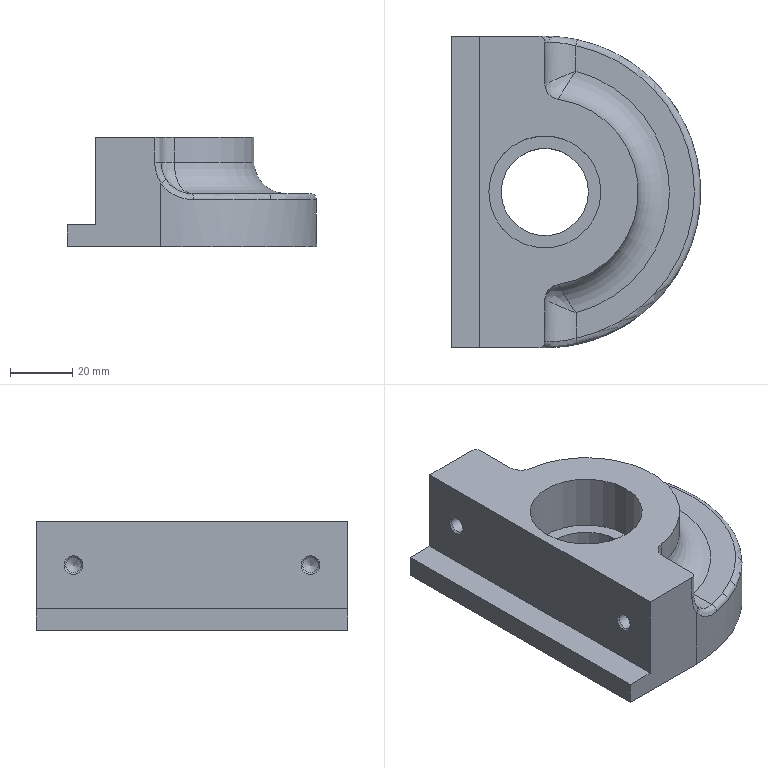Part | NX | features BLEND 3, DATUM_CSYS 2, EXTRUDE 2, HOLE PACKAGE 2, SIMPLE HOLE 2, SYMBOLIC_THREAD 2, BLOCK 1, CBORE_HOLE 1, DELETE FACE 1, SKETCH 1, SWP104 1 | 1 solid | 35 faces | box 80 x 100 x 35 mm | volume 145409 mm3 | cylinder 12 | plane 11 | spline 4 | torus 4 | cone 4 | commonest cylinder face diameters 4 x2 5 x2 10 x2 20 x2 28 x1 36 x1
STEP:
#1=CARTESIAN_POINT('',(0.,50.,0.));
#2=VERTEX_POINT('',#1);
#3=CARTESIAN_POINT('',(0.,50.,20.367));
#4=VERTEX_POINT('',#3);
#5=CARTESIAN_POINT('',(0.,50.,0.));
#6=DIRECTION('',(0.,0.,1.));
#7=VECTOR('',#6,1000.);
#8=LINE('',#5,#7);
#9=EDGE_CURVE('',#2,#4,#8,.T.);
#10=ORIENTED_EDGE('',*,*,#9,.T.);
#11=CARTESIAN_POINT('',(10.417,48.903,15.));
#12=VERTEX_POINT('',#11);
#13=CARTESIAN_POINT('',(0.,50.,20.367));
#14=CARTESIAN_POINT('',(1.172,50.,18.67));
#15=CARTESIAN_POINT('',(4.364,49.914,15.947));
#16=CARTESIAN_POINT('',(8.401,49.332,15.));
#17=CARTESIAN_POINT('',(10.417,48.903,15.));
#18=B_SPLINE_CURVE_WITH_KNOTS('',3,(#13,#14,#15,#16,#17),.UNSPECIFIED.,.F.,.F.,(4,1,4),(0.,0.006104,0.01221),.UNSPECIFIED.);
#19=EDGE_CURVE('',#4,#12,#18,.T.);
#20=ORIENTED_EDGE('',*,*,#19,.T.);
#21=CARTESIAN_POINT('',(10.417,-48.903,15.));
#22=VERTEX_POINT('',#21);
#23=CARTESIAN_POINT('',(0.,0.,15.));
#24=DIRECTION('',(0.,0.,1.));
#25=DIRECTION('',(1.,0.,0.));
#26=AXIS2_PLACEMENT_3D('',#23,#24,#25);
#27=CIRCLE('',#26,50.);
#28=EDGE_CURVE('',#12,#22,#27,.F.);
#29=ORIENTED_EDGE('',*,*,#28,.T.);
#30=CARTESIAN_POINT('',(0.,-50.,20.367));
#31=VERTEX_POINT('',#30);
#32=CARTESIAN_POINT('',(10.417,-48.903,15.));
#33=CARTESIAN_POINT('',(8.401,-49.332,15.));
#34=CARTESIAN_POINT('',(4.364,-49.914,15.947));
#35=CARTESIAN_POINT('',(1.172,-50.,18.67));
#36=CARTESIAN_POINT('',(0.,-50.,20.367));
#37=B_SPLINE_CURVE_WITH_KNOTS('',3,(#32,#33,#34,#35,#36),.UNSPECIFIED.,.F.,.F.,(4,1,4),(0.,0.006102,0.0122),.UNSPECIFIED.);
#38=EDGE_CURVE('',#22,#31,#37,.T.);
#39=ORIENTED_EDGE('',*,*,#38,.T.);
#40=CARTESIAN_POINT('',(0.,-50.,0.));
#41=VERTEX_POINT('',#40);
#42=CARTESIAN_POINT('',(0.,-50.,0.));
#43=DIRECTION('',(0.,0.,1.));
#44=VECTOR('',#43,1000.);
#45=LINE('',#42,#44);
#46=EDGE_CURVE('',#41,#31,#45,.T.);
#47=ORIENTED_EDGE('',*,*,#46,.F.);
#48=CARTESIAN_POINT('',(0.,0.,0.));
#49=DIRECTION('',(0.,0.,1.));
#50=DIRECTION('',(1.,0.,0.));
#51=AXIS2_PLACEMENT_3D('',#48,#49,#50);
#52=CIRCLE('',#51,50.);
#53=EDGE_CURVE('',#41,#2,#52,.T.);
#54=ORIENTED_EDGE('',*,*,#53,.T.);
#55=EDGE_LOOP('',(#10,#20,#29,#39,#47,#54));
#56=FACE_BOUND('',#55,.T.);
#57=CARTESIAN_POINT('',(0.,0.,0.));
#58=DIRECTION('',(0.,0.,1.));
#59=DIRECTION('',(1.,0.,0.));
#60=AXIS2_PLACEMENT_3D('',#57,#58,#59);
#61=CYLINDRICAL_SURFACE('',#60,50.);
#62=ADVANCED_FACE('',(#56),#61,.T.);
#63=CARTESIAN_POINT('',(-18.,0.,35.));
#64=VERTEX_POINT('',#63);
#65=CARTESIAN_POINT('',(0.,0.,35.));
#66=DIRECTION('',(0.,0.,-1.));
#67=DIRECTION('',(-1.,0.,0.));
#68=AXIS2_PLACEMENT_3D('',#65,#66,#67);
#69=CIRCLE('',#68,18.);
#70=EDGE_CURVE('',#64,#64,#69,.T.);
#71=ORIENTED_EDGE('',*,*,#70,.T.);
#72=EDGE_LOOP('',(#71));
#73=FACE_BOUND('',#72,.T.);
#74=CARTESIAN_POINT('',(-2.,-50.,35.));
#75=VERTEX_POINT('',#74);
#76=CARTESIAN_POINT('',(-21.,-50.,35.));
#77=VERTEX_POINT('',#76);
#78=CARTESIAN_POINT('',(-15.,-50.,35.));
#79=DIRECTION('',(-1.,0.,0.));
#80=VECTOR('',#79,1000.);
#81=LINE('',#78,#80);
#82=EDGE_CURVE('',#75,#77,#81,.T.);
#83=ORIENTED_EDGE('',*,*,#82,.F.);
#84=CARTESIAN_POINT('',(0.,-48.,35.));
#85=VERTEX_POINT('',#84);
#86=CARTESIAN_POINT('',(-2.,-48.,35.));
#87=DIRECTION('',(0.,0.,1.));
#88=DIRECTION('',(1.,0.,0.));
#89=AXIS2_PLACEMENT_3D('',#86,#87,#88);
#90=CIRCLE('',#89,2.);
#91=EDGE_CURVE('',#75,#85,#90,.T.);
#92=ORIENTED_EDGE('',*,*,#91,.T.);
#93=CARTESIAN_POINT('',(0.,-34.641,35.));
#94=VERTEX_POINT('',#93);
#95=CARTESIAN_POINT('',(0.,-50.,35.));
#96=DIRECTION('',(0.,-1.,0.));
#97=VECTOR('',#96,1000.);
#98=LINE('',#95,#97);
#99=EDGE_CURVE('',#85,#94,#98,.F.);
#100=ORIENTED_EDGE('',*,*,#99,.T.);
#101=CARTESIAN_POINT('',(4.286,-29.692,35.));
#102=VERTEX_POINT('',#101);
#103=CARTESIAN_POINT('',(5.,-34.641,35.));
#104=DIRECTION('',(0.,0.,1.));
#105=DIRECTION('',(1.,0.,0.));
#106=AXIS2_PLACEMENT_3D('',#103,#104,#105);
#107=CIRCLE('',#106,5.);
#108=EDGE_CURVE('',#94,#102,#107,.F.);
#109=ORIENTED_EDGE('',*,*,#108,.T.);
#110=CARTESIAN_POINT('',(4.286,29.692,35.));
#111=VERTEX_POINT('',#110);
#112=CARTESIAN_POINT('',(0.,0.,35.));
#113=DIRECTION('',(0.,0.,-1.));
#114=DIRECTION('',(-1.,0.,0.));
#115=AXIS2_PLACEMENT_3D('',#112,#113,#114);
#116=CIRCLE('',#115,30.);
#117=EDGE_CURVE('',#111,#102,#116,.T.);
#118=ORIENTED_EDGE('',*,*,#117,.F.);
#119=CARTESIAN_POINT('',(0.,34.641,35.));
#120=VERTEX_POINT('',#119);
#121=CARTESIAN_POINT('',(5.,34.641,35.));
#122=DIRECTION('',(0.,0.,1.));
#123=DIRECTION('',(1.,0.,0.));
#124=AXIS2_PLACEMENT_3D('',#121,#122,#123);
#125=CIRCLE('',#124,5.);
#126=EDGE_CURVE('',#111,#120,#125,.F.);
#127=ORIENTED_EDGE('',*,*,#126,.T.);
#128=CARTESIAN_POINT('',(0.,48.,35.));
#129=VERTEX_POINT('',#128);
#130=CARTESIAN_POINT('',(0.,50.,35.));
#131=DIRECTION('',(0.,1.,0.));
#132=VECTOR('',#131,1000.);
#133=LINE('',#130,#132);
#134=EDGE_CURVE('',#129,#120,#133,.F.);
#135=ORIENTED_EDGE('',*,*,#134,.F.);
#136=CARTESIAN_POINT('',(-2.,50.,35.));
#137=VERTEX_POINT('',#136);
#138=CARTESIAN_POINT('',(-2.,48.,35.));
#139=DIRECTION('',(0.,0.,1.));
#140=DIRECTION('',(1.,0.,0.));
#141=AXIS2_PLACEMENT_3D('',#138,#139,#140);
#142=CIRCLE('',#141,2.);
#143=EDGE_CURVE('',#129,#137,#142,.T.);
#144=ORIENTED_EDGE('',*,*,#143,.T.);
#145=CARTESIAN_POINT('',(-21.,50.,35.));
#146=VERTEX_POINT('',#145);
#147=CARTESIAN_POINT('',(-15.,50.,35.));
#148=DIRECTION('',(1.,0.,0.));
#149=VECTOR('',#148,1000.);
#150=LINE('',#147,#149);
#151=EDGE_CURVE('',#146,#137,#150,.T.);
#152=ORIENTED_EDGE('',*,*,#151,.F.);
#153=CARTESIAN_POINT('',(-21.,50.,35.));
#154=DIRECTION('',(0.,1.,0.));
#155=VECTOR('',#154,1000.);
#156=LINE('',#153,#155);
#157=EDGE_CURVE('',#146,#77,#156,.F.);
#158=ORIENTED_EDGE('',*,*,#157,.T.);
#159=EDGE_LOOP('',(#83,#92,#100,#109,#118,#127,#135,#144,#152,#158));
#160=FACE_BOUND('',#159,.T.);
#161=CARTESIAN_POINT('',(-15.,0.,35.));
#162=DIRECTION('',(0.,0.,1.));
#163=DIRECTION('',(1.,0.,0.));
#164=AXIS2_PLACEMENT_3D('',#161,#162,#163);
#165=PLANE('',#164);
#166=ADVANCED_FACE('',(#73,#160),#165,.T.);
#167=CARTESIAN_POINT('',(-2.,-50.,27.));
#168=VERTEX_POINT('',#167);
#169=CARTESIAN_POINT('',(10.,-50.,27.));
#170=DIRECTION('',(0.,-1.,0.));
#171=DIRECTION('',(0.,0.,-1.));
#172=AXIS2_PLACEMENT_3D('',#169,#170,#171);
#173=CIRCLE('',#172,12.);
#174=EDGE_CURVE('',#31,#168,#173,.F.);
#175=ORIENTED_EDGE('',*,*,#174,.T.);
#176=CARTESIAN_POINT('',(-2.,-50.,0.));
#177=DIRECTION('',(0.,0.,1.));
#178=VECTOR('',#177,1000.);
#179=LINE('',#176,#178);
#180=EDGE_CURVE('',#168,#75,#179,.T.);
#181=ORIENTED_EDGE('',*,*,#180,.T.);
#182=ORIENTED_EDGE('',*,*,#82,.T.);
#183=CARTESIAN_POINT('',(-21.,-50.,7.));
#184=VERTEX_POINT('',#183);
#185=CARTESIAN_POINT('',(-21.,-50.,35.));
#186=DIRECTION('',(0.,0.,-1.));
#187=VECTOR('',#186,1000.);
#188=LINE('',#185,#187);
#189=EDGE_CURVE('',#77,#184,#188,.T.);
#190=ORIENTED_EDGE('',*,*,#189,.T.);
#191=CARTESIAN_POINT('',(-30.,-50.,7.));
#192=VERTEX_POINT('',#191);
#193=CARTESIAN_POINT('',(-30.,-50.,7.));
#194=DIRECTION('',(1.,0.,0.));
#195=VECTOR('',#194,1000.);
#196=LINE('',#193,#195);
#197=EDGE_CURVE('',#192,#184,#196,.T.);
#198=ORIENTED_EDGE('',*,*,#197,.F.);
#199=CARTESIAN_POINT('',(-30.,-50.,0.));
#200=VERTEX_POINT('',#199);
#201=CARTESIAN_POINT('',(-30.,-50.,0.));
#202=DIRECTION('',(0.,0.,1.));
#203=VECTOR('',#202,1000.);
#204=LINE('',#201,#203);
#205=EDGE_CURVE('',#200,#192,#204,.T.);
#206=ORIENTED_EDGE('',*,*,#205,.F.);
#207=CARTESIAN_POINT('',(-15.,-50.,0.));
#208=DIRECTION('',(1.,0.,0.));
#209=VECTOR('',#208,1000.);
#210=LINE('',#207,#209);
#211=EDGE_CURVE('',#200,#41,#210,.T.);
#212=ORIENTED_EDGE('',*,*,#211,.T.);
#213=ORIENTED_EDGE('',*,*,#46,.T.);
#214=EDGE_LOOP('',(#175,#181,#182,#190,#198,#206,#212,#213));
#215=FACE_BOUND('',#214,.T.);
#216=CARTESIAN_POINT('',(-15.,-50.,0.));
#217=DIRECTION('',(0.,-1.,0.));
#218=DIRECTION('',(0.,0.,-1.));
#219=AXIS2_PLACEMENT_3D('',#216,#217,#218);
#220=PLANE('',#219);
#221=ADVANCED_FACE('',(#215),#220,.T.);
#222=CARTESIAN_POINT('',(-30.,50.,7.));
#223=VERTEX_POINT('',#222);
#224=CARTESIAN_POINT('',(-30.,50.,7.));
#225=DIRECTION('',(0.,-1.,0.));
#226=VECTOR('',#225,1000.);
#227=LINE('',#224,#226);
#228=EDGE_CURVE('',#223,#192,#227,.T.);
#229=ORIENTED_EDGE('',*,*,#228,.F.);
#230=CARTESIAN_POINT('',(-30.,50.,0.));
#231=VERTEX_POINT('',#230);
#232=CARTESIAN_POINT('',(-30.,50.,0.));
#233=DIRECTION('',(0.,0.,1.));
#234=VECTOR('',#233,1000.);
#235=LINE('',#232,#234);
#236=EDGE_CURVE('',#231,#223,#235,.T.);
#237=ORIENTED_EDGE('',*,*,#236,.F.);
#238=CARTESIAN_POINT('',(-30.,0.,0.));
#239=DIRECTION('',(0.,-1.,0.));
#240=VECTOR('',#239,1000.);
#241=LINE('',#238,#240);
#242=EDGE_CURVE('',#231,#200,#241,.T.);
#243=ORIENTED_EDGE('',*,*,#242,.T.);
#244=ORIENTED_EDGE('',*,*,#205,.T.);
#245=EDGE_LOOP('',(#229,#237,#243,#244));
#246=FACE_BOUND('',#245,.T.);
#247=CARTESIAN_POINT('',(-30.,0.,0.));
#248=DIRECTION('',(-1.,0.,0.));
#249=DIRECTION('',(0.,0.,1.));
#250=AXIS2_PLACEMENT_3D('',#247,#248,#249);
#251=PLANE('',#250);
#252=ADVANCED_FACE('',(#246),#251,.T.);
#253=ORIENTED_EDGE('',*,*,#151,.T.);
#254=CARTESIAN_POINT('',(-2.,50.,27.));
#255=VERTEX_POINT('',#254);
#256=CARTESIAN_POINT('',(-2.,50.,0.));
#257=DIRECTION('',(0.,0.,-1.));
#258=VECTOR('',#257,1000.);
#259=LINE('',#256,#258);
#260=EDGE_CURVE('',#137,#255,#259,.T.);
#261=ORIENTED_EDGE('',*,*,#260,.T.);
#262=CARTESIAN_POINT('',(10.,50.,27.));
#263=DIRECTION('',(0.,1.,0.));
#264=DIRECTION('',(0.,0.,1.));
#265=AXIS2_PLACEMENT_3D('',#262,#263,#264);
#266=CIRCLE('',#265,12.);
#267=EDGE_CURVE('',#255,#4,#266,.F.);
#268=ORIENTED_EDGE('',*,*,#267,.T.);
#269=ORIENTED_EDGE('',*,*,#9,.F.);
#270=CARTESIAN_POINT('',(-15.,50.,0.));
#271=DIRECTION('',(-1.,0.,0.));
#272=VECTOR('',#271,1000.);
#273=LINE('',#270,#272);
#274=EDGE_CURVE('',#2,#231,#273,.T.);
#275=ORIENTED_EDGE('',*,*,#274,.T.);
#276=ORIENTED_EDGE('',*,*,#236,.T.);
#277=CARTESIAN_POINT('',(-21.,50.,7.));
#278=VERTEX_POINT('',#277);
#279=CARTESIAN_POINT('',(-30.,50.,7.));
#280=DIRECTION('',(1.,0.,0.));
#281=VECTOR('',#280,1000.);
#282=LINE('',#279,#281);
#283=EDGE_CURVE('',#223,#278,#282,.T.);
#284=ORIENTED_EDGE('',*,*,#283,.T.);
#285=CARTESIAN_POINT('',(-21.,50.,35.));
#286=DIRECTION('',(0.,0.,-1.));
#287=VECTOR('',#286,1000.);
#288=LINE('',#285,#287);
#289=EDGE_CURVE('',#146,#278,#288,.T.);
#290=ORIENTED_EDGE('',*,*,#289,.F.);
#291=EDGE_LOOP('',(#253,#261,#268,#269,#275,#276,#284,#290));
#292=FACE_BOUND('',#291,.T.);
#293=CARTESIAN_POINT('',(-15.,50.,0.));
#294=DIRECTION('',(0.,1.,0.));
#295=DIRECTION('',(0.,0.,1.));
#296=AXIS2_PLACEMENT_3D('',#293,#294,#295);
#297=PLANE('',#296);
#298=ADVANCED_FACE('',(#292),#297,.T.);
#299=CARTESIAN_POINT('',(-14.,0.,0.));
#300=VERTEX_POINT('',#299);
#301=CARTESIAN_POINT('',(0.,0.,0.));
#302=DIRECTION('',(0.,0.,-1.));
#303=DIRECTION('',(-1.,0.,0.));
#304=AXIS2_PLACEMENT_3D('',#301,#302,#303);
#305=CIRCLE('',#304,14.);
#306=EDGE_CURVE('',#300,#300,#305,.T.);
#307=ORIENTED_EDGE('',*,*,#306,.F.);
#308=EDGE_LOOP('',(#307));
#309=FACE_BOUND('',#308,.T.);
#310=ORIENTED_EDGE('',*,*,#211,.F.);
#311=ORIENTED_EDGE('',*,*,#242,.F.);
#312=ORIENTED_EDGE('',*,*,#274,.F.);
#313=ORIENTED_EDGE('',*,*,#53,.F.);
#314=EDGE_LOOP('',(#310,#311,#312,#313));
#315=FACE_BOUND('',#314,.T.);
#316=CARTESIAN_POINT('',(-15.,0.,0.));
#317=DIRECTION('',(0.,0.,-1.));
#318=DIRECTION('',(-1.,0.,0.));
#319=AXIS2_PLACEMENT_3D('',#316,#317,#318);
#320=PLANE('',#319);
#321=ADVANCED_FACE('',(#309,#315),#320,.T.);
#322=ORIENTED_EDGE('',*,*,#197,.T.);
#323=CARTESIAN_POINT('',(-21.,50.,7.));
#324=DIRECTION('',(0.,1.,0.));
#325=VECTOR('',#324,1000.);
#326=LINE('',#323,#325);
#327=EDGE_CURVE('',#184,#278,#326,.T.);
#328=ORIENTED_EDGE('',*,*,#327,.T.);
#329=ORIENTED_EDGE('',*,*,#283,.F.);
#330=ORIENTED_EDGE('',*,*,#228,.T.);
#331=EDGE_LOOP('',(#322,#328,#329,#330));
#332=FACE_BOUND('',#331,.T.);
#333=CARTESIAN_POINT('',(-30.,50.,7.));
#334=DIRECTION('',(0.,0.,1.));
#335=DIRECTION('',(0.,-1.,0.));
#336=AXIS2_PLACEMENT_3D('',#333,#334,#335);
#337=PLANE('',#336);
#338=ADVANCED_FACE('',(#332),#337,.T.);
#339=CARTESIAN_POINT('',(-21.,38.,18.));
#340=VERTEX_POINT('',#339);
#341=CARTESIAN_POINT('',(-21.,38.,21.));
#342=DIRECTION('',(1.,0.,0.));
#343=DIRECTION('',(0.,0.,-1.));
#344=AXIS2_PLACEMENT_3D('',#341,#342,#343);
#345=CIRCLE('',#344,3.);
#346=EDGE_CURVE('',#340,#340,#345,.T.);
#347=ORIENTED_EDGE('',*,*,#346,.T.);
#348=EDGE_LOOP('',(#347));
#349=FACE_BOUND('',#348,.T.);
#350=CARTESIAN_POINT('',(-21.,-38.,18.));
#351=VERTEX_POINT('',#350);
#352=CARTESIAN_POINT('',(-21.,-38.,21.));
#353=DIRECTION('',(1.,0.,0.));
#354=DIRECTION('',(0.,0.,-1.));
#355=AXIS2_PLACEMENT_3D('',#352,#353,#354);
#356=CIRCLE('',#355,3.);
#357=EDGE_CURVE('',#351,#351,#356,.T.);
#358=ORIENTED_EDGE('',*,*,#357,.T.);
#359=EDGE_LOOP('',(#358));
#360=FACE_BOUND('',#359,.T.);
#361=ORIENTED_EDGE('',*,*,#327,.F.);
#362=ORIENTED_EDGE('',*,*,#189,.F.);
#363=ORIENTED_EDGE('',*,*,#157,.F.);
#364=ORIENTED_EDGE('',*,*,#289,.T.);
#365=EDGE_LOOP('',(#361,#362,#363,#364));
#366=FACE_BOUND('',#365,.T.);
#367=CARTESIAN_POINT('',(-21.,50.,35.));
#368=DIRECTION('',(1.,0.,0.));
#369=DIRECTION('',(0.,0.,-1.));
#370=AXIS2_PLACEMENT_3D('',#367,#368,#369);
#371=PLANE('',#370);
#372=ADVANCED_FACE('',(#349,#360,#366),#371,.F.);
#373=ORIENTED_EDGE('',*,*,#99,.F.);
#374=CARTESIAN_POINT('',(0.,-48.,27.));
#375=VERTEX_POINT('',#374);
#376=CARTESIAN_POINT('',(0.,-48.,26.));
#377=DIRECTION('',(0.,0.,-1.));
#378=VECTOR('',#377,1000.);
#379=LINE('',#376,#378);
#380=EDGE_CURVE('',#85,#375,#379,.T.);
#381=ORIENTED_EDGE('',*,*,#380,.T.);
#382=CARTESIAN_POINT('',(0.,-34.641,27.));
#383=VERTEX_POINT('',#382);
#384=CARTESIAN_POINT('',(0.,-34.641,27.));
#385=DIRECTION('',(0.,-1.,0.));
#386=VECTOR('',#385,1000.);
#387=LINE('',#384,#386);
#388=EDGE_CURVE('',#375,#383,#387,.F.);
#389=ORIENTED_EDGE('',*,*,#388,.T.);
#390=CARTESIAN_POINT('',(0.,-34.641,35.));
#391=DIRECTION('',(0.,0.,-1.));
#392=VECTOR('',#391,1000.);
#393=LINE('',#390,#392);
#394=EDGE_CURVE('',#383,#94,#393,.F.);
#395=ORIENTED_EDGE('',*,*,#394,.T.);
#396=EDGE_LOOP('',(#373,#381,#389,#395));
#397=FACE_BOUND('',#396,.T.);
#398=CARTESIAN_POINT('',(0.,-50.,26.));
#399=DIRECTION('',(-1.,0.,0.));
#400=DIRECTION('',(0.,0.,-1.));
#401=AXIS2_PLACEMENT_3D('',#398,#399,#400);
#402=PLANE('',#401);
#403=ADVANCED_FACE('',(#397),#402,.F.);
#404=CARTESIAN_POINT('',(10.,-38.73,17.));
#405=VERTEX_POINT('',#404);
#406=CARTESIAN_POINT('',(10.,-46.947,17.));
#407=VERTEX_POINT('',#406);
#408=CARTESIAN_POINT('',(10.,-50.,17.));
#409=DIRECTION('',(0.,1.,0.));
#410=VECTOR('',#409,1000.);
#411=LINE('',#408,#410);
#412=EDGE_CURVE('',#405,#407,#411,.F.);
#413=ORIENTED_EDGE('',*,*,#412,.T.);
#414=CARTESIAN_POINT('',(10.,46.947,17.));
#415=VERTEX_POINT('',#414);
#416=CARTESIAN_POINT('',(0.,0.,17.));
#417=DIRECTION('',(0.,0.,1.));
#418=DIRECTION('',(1.,0.,0.));
#419=AXIS2_PLACEMENT_3D('',#416,#417,#418);
#420=CIRCLE('',#419,48.);
#421=EDGE_CURVE('',#407,#415,#420,.T.);
#422=ORIENTED_EDGE('',*,*,#421,.T.);
#423=CARTESIAN_POINT('',(10.,38.73,17.));
#424=VERTEX_POINT('',#423);
#425=CARTESIAN_POINT('',(10.,34.641,17.));
#426=DIRECTION('',(0.,1.,0.));
#427=VECTOR('',#426,1000.);
#428=LINE('',#425,#427);
#429=EDGE_CURVE('',#415,#424,#428,.F.);
#430=ORIENTED_EDGE('',*,*,#429,.T.);
#431=CARTESIAN_POINT('',(0.,0.,17.));
#432=DIRECTION('',(0.,0.,1.));
#433=DIRECTION('',(1.,0.,0.));
#434=AXIS2_PLACEMENT_3D('',#431,#432,#433);
#435=CIRCLE('',#434,40.);
#436=EDGE_CURVE('',#424,#405,#435,.F.);
#437=ORIENTED_EDGE('',*,*,#436,.T.);
#438=EDGE_LOOP('',(#413,#422,#430,#437));
#439=FACE_BOUND('',#438,.T.);
#440=CARTESIAN_POINT('',(0.,0.,17.));
#441=DIRECTION('',(0.,0.,1.));
#442=DIRECTION('',(1.,0.,0.));
#443=AXIS2_PLACEMENT_3D('',#440,#441,#442);
#444=PLANE('',#443);
#445=ADVANCED_FACE('',(#439),#444,.T.);
#446=CARTESIAN_POINT('',(0.,34.641,27.));
#447=VERTEX_POINT('',#446);
#448=CARTESIAN_POINT('',(0.,48.,27.));
#449=VERTEX_POINT('',#448);
#450=CARTESIAN_POINT('',(0.,50.,27.));
#451=DIRECTION('',(0.,1.,0.));
#452=VECTOR('',#451,1000.);
#453=LINE('',#450,#452);
#454=EDGE_CURVE('',#447,#449,#453,.T.);
#455=ORIENTED_EDGE('',*,*,#454,.T.);
#456=CARTESIAN_POINT('',(0.,48.,26.));
#457=DIRECTION('',(0.,0.,-1.));
#458=VECTOR('',#457,1000.);
#459=LINE('',#456,#458);
#460=EDGE_CURVE('',#449,#129,#459,.F.);
#461=ORIENTED_EDGE('',*,*,#460,.T.);
#462=ORIENTED_EDGE('',*,*,#134,.T.);
#463=CARTESIAN_POINT('',(0.,34.641,17.));
#464=DIRECTION('',(0.,0.,1.));
#465=VECTOR('',#464,1000.);
#466=LINE('',#463,#465);
#467=EDGE_CURVE('',#120,#447,#466,.F.);
#468=ORIENTED_EDGE('',*,*,#467,.T.);
#469=EDGE_LOOP('',(#455,#461,#462,#468));
#470=FACE_BOUND('',#469,.T.);
#471=CARTESIAN_POINT('',(0.,50.,26.));
#472=DIRECTION('',(1.,0.,0.));
#473=DIRECTION('',(0.,0.,-1.));
#474=AXIS2_PLACEMENT_3D('',#471,#472,#473);
#475=PLANE('',#474);
#476=ADVANCED_FACE('',(#470),#475,.T.);
#477=CARTESIAN_POINT('',(4.286,-29.692,27.));
#478=VERTEX_POINT('',#477);
#479=CARTESIAN_POINT('',(4.286,-29.692,35.));
#480=DIRECTION('',(0.,0.,-1.));
#481=VECTOR('',#480,1000.);
#482=LINE('',#479,#481);
#483=EDGE_CURVE('',#102,#478,#482,.T.);
#484=ORIENTED_EDGE('',*,*,#483,.T.);
#485=CARTESIAN_POINT('',(4.286,29.692,27.));
#486=VERTEX_POINT('',#485);
#487=CARTESIAN_POINT('',(0.,0.,27.));
#488=DIRECTION('',(0.,0.,1.));
#489=DIRECTION('',(1.,0.,0.));
#490=AXIS2_PLACEMENT_3D('',#487,#488,#489);
#491=CIRCLE('',#490,30.);
#492=EDGE_CURVE('',#478,#486,#491,.T.);
#493=ORIENTED_EDGE('',*,*,#492,.T.);
#494=CARTESIAN_POINT('',(4.286,29.692,35.));
#495=DIRECTION('',(0.,0.,-1.));
#496=VECTOR('',#495,1000.);
#497=LINE('',#494,#496);
#498=EDGE_CURVE('',#486,#111,#497,.F.);
#499=ORIENTED_EDGE('',*,*,#498,.T.);
#500=ORIENTED_EDGE('',*,*,#117,.T.);
#501=EDGE_LOOP('',(#484,#493,#499,#500));
#502=FACE_BOUND('',#501,.T.);
#503=CARTESIAN_POINT('',(0.,0.,35.));
#504=DIRECTION('',(0.,0.,-1.));
#505=DIRECTION('',(-1.,0.,0.));
#506=AXIS2_PLACEMENT_3D('',#503,#504,#505);
#507=CYLINDRICAL_SURFACE('',#506,30.);
#508=ADVANCED_FACE('',(#502),#507,.T.);
#509=ORIENTED_EDGE('',*,*,#306,.T.);
#510=EDGE_LOOP('',(#509));
#511=FACE_BOUND('',#510,.T.);
#512=CARTESIAN_POINT('',(-14.,0.,17.));
#513=VERTEX_POINT('',#512);
#514=CARTESIAN_POINT('',(0.,0.,17.));
#515=DIRECTION('',(0.,0.,-1.));
#516=DIRECTION('',(-1.,0.,0.));
#517=AXIS2_PLACEMENT_3D('',#514,#515,#516);
#518=CIRCLE('',#517,14.);
#519=EDGE_CURVE('',#513,#513,#518,.F.);
#520=ORIENTED_EDGE('',*,*,#519,.T.);
#521=EDGE_LOOP('',(#520));
#522=FACE_BOUND('',#521,.T.);
#523=CARTESIAN_POINT('',(0.,0.,-54.83));
#524=DIRECTION('',(0.,0.,-1.));
#525=DIRECTION('',(-1.,0.,0.));
#526=AXIS2_PLACEMENT_3D('',#523,#524,#525);
#527=CYLINDRICAL_SURFACE('',#526,14.);
#528=ADVANCED_FACE('',(#511,#522),#527,.F.);
#529=ORIENTED_EDGE('',*,*,#519,.F.);
#530=EDGE_LOOP('',(#529));
#531=FACE_BOUND('',#530,.T.);
#532=CARTESIAN_POINT('',(-18.,0.,17.));
#533=VERTEX_POINT('',#532);
#534=CARTESIAN_POINT('',(0.,0.,17.));
#535=DIRECTION('',(0.,0.,-1.));
#536=DIRECTION('',(-1.,0.,0.));
#537=AXIS2_PLACEMENT_3D('',#534,#535,#536);
#538=CIRCLE('',#537,18.);
#539=EDGE_CURVE('',#533,#533,#538,.F.);
#540=ORIENTED_EDGE('',*,*,#539,.T.);
#541=EDGE_LOOP('',(#540));
#542=FACE_BOUND('',#541,.T.);
#543=CARTESIAN_POINT('',(0.,0.,17.));
#544=DIRECTION('',(0.,0.,-1.));
#545=DIRECTION('',(-1.,0.,0.));
#546=AXIS2_PLACEMENT_3D('',#543,#544,#545);
#547=PLANE('',#546);
#548=ADVANCED_FACE('',(#531,#542),#547,.F.);
#549=ORIENTED_EDGE('',*,*,#539,.F.);
#550=EDGE_LOOP('',(#549));
#551=FACE_BOUND('',#550,.T.);
#552=ORIENTED_EDGE('',*,*,#70,.F.);
#553=EDGE_LOOP('',(#552));
#554=FACE_BOUND('',#553,.T.);
#555=CARTESIAN_POINT('',(0.,0.,35.));
#556=DIRECTION('',(0.,0.,-1.));
#557=DIRECTION('',(-1.,0.,0.));
#558=AXIS2_PLACEMENT_3D('',#555,#556,#557);
#559=CYLINDRICAL_SURFACE('',#558,18.);
#560=ADVANCED_FACE('',(#551,#554),#559,.F.);
#561=ORIENTED_EDGE('',*,*,#394,.F.);
#562=CARTESIAN_POINT('',(5.,-34.641,27.));
#563=DIRECTION('',(0.,0.,-1.));
#564=DIRECTION('',(-1.,0.,0.));
#565=AXIS2_PLACEMENT_3D('',#562,#563,#564);
#566=CIRCLE('',#565,5.);
#567=EDGE_CURVE('',#383,#478,#566,.T.);
#568=ORIENTED_EDGE('',*,*,#567,.T.);
#569=ORIENTED_EDGE('',*,*,#483,.F.);
#570=ORIENTED_EDGE('',*,*,#108,.F.);
#571=EDGE_LOOP('',(#561,#568,#569,#570));
#572=FACE_BOUND('',#571,.T.);
#573=CARTESIAN_POINT('',(5.,-34.641,35.));
#574=DIRECTION('',(0.,0.,-1.));
#575=DIRECTION('',(-1.,0.,0.));
#576=AXIS2_PLACEMENT_3D('',#573,#574,#575);
#577=CYLINDRICAL_SURFACE('',#576,5.);
#578=ADVANCED_FACE('',(#572),#577,.F.);
#579=ORIENTED_EDGE('',*,*,#498,.F.);
#580=CARTESIAN_POINT('',(5.,34.641,27.));
#581=DIRECTION('',(0.,0.,-1.));
#582=DIRECTION('',(-1.,0.,0.));
#583=AXIS2_PLACEMENT_3D('',#580,#581,#582);
#584=CIRCLE('',#583,5.);
#585=EDGE_CURVE('',#486,#447,#584,.T.);
#586=ORIENTED_EDGE('',*,*,#585,.T.);
#587=ORIENTED_EDGE('',*,*,#467,.F.);
#588=ORIENTED_EDGE('',*,*,#126,.F.);
#589=EDGE_LOOP('',(#579,#586,#587,#588));
#590=FACE_BOUND('',#589,.T.);
#591=CARTESIAN_POINT('',(5.,34.641,35.));
#592=DIRECTION('',(0.,0.,-1.));
#593=DIRECTION('',(-1.,0.,0.));
#594=AXIS2_PLACEMENT_3D('',#591,#592,#593);
#595=CYLINDRICAL_SURFACE('',#594,5.);
#596=ADVANCED_FACE('',(#590),#595,.F.);
#597=ORIENTED_EDGE('',*,*,#429,.F.);
#598=CARTESIAN_POINT('',(1.667,48.,21.472));
#599=VERTEX_POINT('',#598);
#600=CARTESIAN_POINT('',(10.,46.947,17.));
#601=CARTESIAN_POINT('',(8.381,47.361,17.));
#602=CARTESIAN_POINT('',(5.123,47.922,17.803));
#603=CARTESIAN_POINT('',(2.591,48.,20.079));
#604=CARTESIAN_POINT('',(1.667,48.,21.472));
#605=B_SPLINE_CURVE_WITH_KNOTS('',3,(#600,#601,#602,#603,#604),.UNSPECIFIED.,.F.,.F.,(4,1,4),(0.,0.004943,0.009887),.UNSPECIFIED.);
#606=EDGE_CURVE('',#415,#599,#605,.T.);
#607=ORIENTED_EDGE('',*,*,#606,.T.);
#608=CARTESIAN_POINT('',(10.,48.,27.));
#609=DIRECTION('',(0.,1.,0.));
#610=DIRECTION('',(0.,0.,1.));
#611=AXIS2_PLACEMENT_3D('',#608,#609,#610);
#612=CIRCLE('',#611,10.);
#613=EDGE_CURVE('',#599,#449,#612,.T.);
#614=ORIENTED_EDGE('',*,*,#613,.T.);
#615=ORIENTED_EDGE('',*,*,#454,.F.);
#616=CARTESIAN_POINT('',(0.,34.641,27.));
#617=CARTESIAN_POINT('',(0.,34.641,24.256));
#618=CARTESIAN_POINT('',(2.37,35.682,18.987));
#619=CARTESIAN_POINT('',(7.47,37.75,17.));
#620=CARTESIAN_POINT('',(10.,38.73,17.));
#621=B_SPLINE_CURVE_WITH_KNOTS('',3,(#616,#617,#618,#619,#620),.UNSPECIFIED.,.F.,.F.,(4,1,4),(0.,0.008138,0.01628),.UNSPECIFIED.);
#622=EDGE_CURVE('',#424,#447,#621,.F.);
#623=ORIENTED_EDGE('',*,*,#622,.F.);
#624=EDGE_LOOP('',(#597,#607,#614,#615,#623));
#625=FACE_BOUND('',#624,.T.);
#626=CARTESIAN_POINT('',(10.,50.,27.));
#627=DIRECTION('',(0.,-1.,0.));
#628=DIRECTION('',(1.,0.,0.));
#629=AXIS2_PLACEMENT_3D('',#626,#627,#628);
#630=CYLINDRICAL_SURFACE('',#629,10.);
#631=ADVANCED_FACE('',(#625),#630,.F.);
#632=ORIENTED_EDGE('',*,*,#622,.T.);
#633=ORIENTED_EDGE('',*,*,#585,.F.);
#634=CARTESIAN_POINT('',(4.286,29.692,27.));
#635=CARTESIAN_POINT('',(4.286,29.692,24.268));
#636=CARTESIAN_POINT('',(5.451,31.92,18.989));
#637=CARTESIAN_POINT('',(8.426,36.534,17.));
#638=CARTESIAN_POINT('',(10.,38.73,17.));
#639=B_SPLINE_CURVE_WITH_KNOTS('',3,(#634,#635,#636,#637,#638),.UNSPECIFIED.,.F.,.F.,(4,1,4),(0.,0.008105,0.01621),.UNSPECIFIED.);
#640=EDGE_CURVE('',#424,#486,#639,.F.);
#641=ORIENTED_EDGE('',*,*,#640,.F.);
#642=EDGE_LOOP('',(#632,#633,#641));
#643=FACE_BOUND('',#642,.T.);
#644=CARTESIAN_POINT('',(0.,34.641,27.));
#645=CARTESIAN_POINT('',(0.,30.311,27.));
#646=CARTESIAN_POINT('',(4.286,29.692,27.));
#647=CARTESIAN_POINT('',(0.,34.641,26.239));
#648=CARTESIAN_POINT('',(0.000000013,30.311,25.953));
#649=CARTESIAN_POINT('',(4.286,29.692,26.239));
#650=CARTESIAN_POINT('',(0.1714,34.715,24.752));
#651=CARTESIAN_POINT('',(0.2998,30.58,23.954));
#652=CARTESIAN_POINT('',(4.373,29.853,24.752));
#653=CARTESIAN_POINT('',(1.144,35.135,21.978));
#654=CARTESIAN_POINT('',(1.779,31.901,20.752));
#655=CARTESIAN_POINT('',(4.874,30.762,21.978));
#656=CARTESIAN_POINT('',(3.245,36.025,19.304));
#657=CARTESIAN_POINT('',(4.201,34.022,18.526));
#658=CARTESIAN_POINT('',(5.994,32.706,19.304));
#659=CARTESIAN_POINT('',(6.439,37.334,17.426));
#660=CARTESIAN_POINT('',(7.079,36.429,17.269));
#661=CARTESIAN_POINT('',(7.815,35.599,17.426));
#662=CARTESIAN_POINT('',(8.816,38.271,17.));
#663=CARTESIAN_POINT('',(9.038,37.985,17.));
#664=CARTESIAN_POINT('',(9.26,37.698,17.));
#665=CARTESIAN_POINT('',(10.,38.73,17.));
#666=CARTESIAN_POINT('',(10.,38.73,17.));
#667=CARTESIAN_POINT('',(10.,38.73,17.));
#668=(BOUNDED_SURFACE()B_SPLINE_SURFACE(3,2,((#644,#645,#646),(#647,#648,#649),(#650,#651,#652),(#653,#654,#655),(#656,#657,#658),(#659,#660,#661),(#662,#663,#664),(#665,#666,#667)),.UNSPECIFIED.,.F.,.F.,.F.)B_SPLINE_SURFACE_WITH_KNOTS((4,1,1,1,1,4),(3,3),(0.,0.001123,0.002246,0.004492,0.006738,0.008984),(0.,1.),.UNSPECIFIED.)GEOMETRIC_REPRESENTATION_ITEM()RATIONAL_B_SPLINE_SURFACE(((1.,0.7559,1.),(1.,0.7559,1.),(1.,0.7666,1.),(1.,0.8212,1.),(1.,0.9112,1.),(1.,0.9837,1.),(1.,1.,1.),(1.,1.,1.)))REPRESENTATION_ITEM('')SURFACE());
#669=ADVANCED_FACE('',(#643),#668,.F.);
#670=ORIENTED_EDGE('',*,*,#640,.T.);
#671=ORIENTED_EDGE('',*,*,#492,.F.);
#672=CARTESIAN_POINT('',(4.286,-29.692,27.));
#673=CARTESIAN_POINT('',(4.286,-29.692,24.268));
#674=CARTESIAN_POINT('',(5.451,-31.92,18.989));
#675=CARTESIAN_POINT('',(8.426,-36.534,17.));
#676=CARTESIAN_POINT('',(10.,-38.73,17.));
#677=B_SPLINE_CURVE_WITH_KNOTS('',3,(#672,#673,#674,#675,#676),.UNSPECIFIED.,.F.,.F.,(4,1,4),(0.,0.008105,0.01621),.UNSPECIFIED.);
#678=EDGE_CURVE('',#405,#478,#677,.F.);
#679=ORIENTED_EDGE('',*,*,#678,.F.);
#680=ORIENTED_EDGE('',*,*,#436,.F.);
#681=EDGE_LOOP('',(#670,#671,#679,#680));
#682=FACE_BOUND('',#681,.T.);
#683=CARTESIAN_POINT('',(0.,0.,27.));
#684=DIRECTION('',(0.,0.,1.));
#685=DIRECTION('',(1.,0.,0.));
#686=AXIS2_PLACEMENT_3D('',#683,#684,#685);
#687=TOROIDAL_SURFACE('',#686,40.,10.);
#688=ADVANCED_FACE('',(#682),#687,.F.);
#689=ORIENTED_EDGE('',*,*,#678,.T.);
#690=ORIENTED_EDGE('',*,*,#567,.F.);
#691=CARTESIAN_POINT('',(0.,-34.641,27.));
#692=CARTESIAN_POINT('',(0.,-34.641,24.256));
#693=CARTESIAN_POINT('',(2.37,-35.682,18.987));
#694=CARTESIAN_POINT('',(7.47,-37.75,17.));
#695=CARTESIAN_POINT('',(10.,-38.73,17.));
#696=B_SPLINE_CURVE_WITH_KNOTS('',3,(#691,#692,#693,#694,#695),.UNSPECIFIED.,.F.,.F.,(4,1,4),(0.,0.008138,0.01628),.UNSPECIFIED.);
#697=EDGE_CURVE('',#405,#383,#696,.F.);
#698=ORIENTED_EDGE('',*,*,#697,.F.);
#699=EDGE_LOOP('',(#689,#690,#698));
#700=FACE_BOUND('',#699,.T.);
#701=CARTESIAN_POINT('',(4.286,-29.692,27.));
#702=CARTESIAN_POINT('',(0.,-30.311,27.));
#703=CARTESIAN_POINT('',(0.,-34.641,27.));
#704=CARTESIAN_POINT('',(4.286,-29.692,26.239));
#705=CARTESIAN_POINT('',(0.000000013,-30.311,25.953));
#706=CARTESIAN_POINT('',(0.,-34.641,26.239));
#707=CARTESIAN_POINT('',(4.373,-29.853,24.752));
#708=CARTESIAN_POINT('',(0.2998,-30.58,23.954));
#709=CARTESIAN_POINT('',(0.1714,-34.715,24.752));
#710=CARTESIAN_POINT('',(4.874,-30.762,21.978));
#711=CARTESIAN_POINT('',(1.779,-31.901,20.752));
#712=CARTESIAN_POINT('',(1.144,-35.135,21.978));
#713=CARTESIAN_POINT('',(5.994,-32.706,19.304));
#714=CARTESIAN_POINT('',(4.201,-34.022,18.526));
#715=CARTESIAN_POINT('',(3.245,-36.025,19.304));
#716=CARTESIAN_POINT('',(7.815,-35.599,17.426));
#717=CARTESIAN_POINT('',(7.079,-36.429,17.269));
#718=CARTESIAN_POINT('',(6.439,-37.334,17.426));
#719=CARTESIAN_POINT('',(9.26,-37.698,17.));
#720=CARTESIAN_POINT('',(9.038,-37.985,17.));
#721=CARTESIAN_POINT('',(8.816,-38.271,17.));
#722=CARTESIAN_POINT('',(10.,-38.73,17.));
#723=CARTESIAN_POINT('',(10.,-38.73,17.));
#724=CARTESIAN_POINT('',(10.,-38.73,17.));
#725=(BOUNDED_SURFACE()B_SPLINE_SURFACE(3,2,((#701,#702,#703),(#704,#705,#706),(#707,#708,#709),(#710,#711,#712),(#713,#714,#715),(#716,#717,#718),(#719,#720,#721),(#722,#723,#724)),.UNSPECIFIED.,.F.,.F.,.F.)B_SPLINE_SURFACE_WITH_KNOTS((4,1,1,1,1,4),(3,3),(0.,0.001123,0.002246,0.004492,0.006738,0.008984),(0.,1.),.UNSPECIFIED.)GEOMETRIC_REPRESENTATION_ITEM()RATIONAL_B_SPLINE_SURFACE(((1.,0.7559,1.),(1.,0.7559,1.),(1.,0.7666,1.),(1.,0.8212,1.),(1.,0.9112,1.),(1.,0.9837,1.),(1.,1.,1.),(1.,1.,1.)))REPRESENTATION_ITEM('')SURFACE());
#726=ADVANCED_FACE('',(#700),#725,.F.);
#727=ORIENTED_EDGE('',*,*,#388,.F.);
#728=CARTESIAN_POINT('',(1.667,-48.,21.472));
#729=VERTEX_POINT('',#728);
#730=CARTESIAN_POINT('',(10.,-48.,27.));
#731=DIRECTION('',(0.,-1.,0.));
#732=DIRECTION('',(0.,0.,-1.));
#733=AXIS2_PLACEMENT_3D('',#730,#731,#732);
#734=CIRCLE('',#733,10.);
#735=EDGE_CURVE('',#375,#729,#734,.T.);
#736=ORIENTED_EDGE('',*,*,#735,.T.);
#737=CARTESIAN_POINT('',(1.667,-48.,21.472));
#738=CARTESIAN_POINT('',(2.591,-48.,20.079));
#739=CARTESIAN_POINT('',(5.123,-47.922,17.803));
#740=CARTESIAN_POINT('',(8.381,-47.361,17.));
#741=CARTESIAN_POINT('',(10.,-46.947,17.));
#742=B_SPLINE_CURVE_WITH_KNOTS('',3,(#737,#738,#739,#740,#741),.UNSPECIFIED.,.F.,.F.,(4,1,4),(0.,0.004948,0.009896),.UNSPECIFIED.);
#743=EDGE_CURVE('',#729,#407,#742,.T.);
#744=ORIENTED_EDGE('',*,*,#743,.T.);
#745=ORIENTED_EDGE('',*,*,#412,.F.);
#746=ORIENTED_EDGE('',*,*,#697,.T.);
#747=EDGE_LOOP('',(#727,#736,#744,#745,#746));
#748=FACE_BOUND('',#747,.T.);
#749=CARTESIAN_POINT('',(10.,0.,27.));
#750=DIRECTION('',(0.,-1.,0.));
#751=DIRECTION('',(1.,0.,0.));
#752=AXIS2_PLACEMENT_3D('',#749,#750,#751);
#753=CYLINDRICAL_SURFACE('',#752,10.);
#754=ADVANCED_FACE('',(#748),#753,.F.);
#755=ORIENTED_EDGE('',*,*,#91,.F.);
#756=ORIENTED_EDGE('',*,*,#180,.F.);
#757=CARTESIAN_POINT('',(-2.,-48.,27.));
#758=DIRECTION('',(0.,0.,-1.));
#759=DIRECTION('',(-1.,0.,0.));
#760=AXIS2_PLACEMENT_3D('',#757,#758,#759);
#761=CIRCLE('',#760,2.);
#762=EDGE_CURVE('',#375,#168,#761,.T.);
#763=ORIENTED_EDGE('',*,*,#762,.F.);
#764=ORIENTED_EDGE('',*,*,#380,.F.);
#765=EDGE_LOOP('',(#755,#756,#763,#764));
#766=FACE_BOUND('',#765,.T.);
#767=CARTESIAN_POINT('',(-2.,-48.,26.));
#768=DIRECTION('',(0.,0.,1.));
#769=DIRECTION('',(1.,0.,0.));
#770=AXIS2_PLACEMENT_3D('',#767,#768,#769);
#771=CYLINDRICAL_SURFACE('',#770,2.);
#772=ADVANCED_FACE('',(#766),#771,.T.);
#773=ORIENTED_EDGE('',*,*,#762,.T.);
#774=ORIENTED_EDGE('',*,*,#174,.F.);
#775=CARTESIAN_POINT('',(0.,-48.,20.367));
#776=DIRECTION('',(0.5528,0.,-0.8333));
#777=DIRECTION('',(-0.8333,0.,-0.5528));
#778=AXIS2_PLACEMENT_3D('',#775,#776,#777);
#779=CIRCLE('',#778,2.);
#780=EDGE_CURVE('',#729,#31,#779,.T.);
#781=ORIENTED_EDGE('',*,*,#780,.F.);
#782=ORIENTED_EDGE('',*,*,#735,.F.);
#783=EDGE_LOOP('',(#773,#774,#781,#782));
#784=FACE_BOUND('',#783,.T.);
#785=CARTESIAN_POINT('',(10.,-48.,27.));
#786=DIRECTION('',(0.,-1.,0.));
#787=DIRECTION('',(0.,0.,-1.));
#788=AXIS2_PLACEMENT_3D('',#785,#786,#787);
#789=TOROIDAL_SURFACE('',#788,12.,2.);
#790=ADVANCED_FACE('',(#784),#789,.T.);
#791=ORIENTED_EDGE('',*,*,#143,.F.);
#792=ORIENTED_EDGE('',*,*,#460,.F.);
#793=CARTESIAN_POINT('',(-2.,48.,27.));
#794=DIRECTION('',(0.,0.,-1.));
#795=DIRECTION('',(-1.,0.,0.));
#796=AXIS2_PLACEMENT_3D('',#793,#794,#795);
#797=CIRCLE('',#796,2.);
#798=EDGE_CURVE('',#255,#449,#797,.T.);
#799=ORIENTED_EDGE('',*,*,#798,.F.);
#800=ORIENTED_EDGE('',*,*,#260,.F.);
#801=EDGE_LOOP('',(#791,#792,#799,#800));
#802=FACE_BOUND('',#801,.T.);
#803=CARTESIAN_POINT('',(-2.,48.,0.));
#804=DIRECTION('',(0.,0.,-1.));
#805=DIRECTION('',(-1.,0.,0.));
#806=AXIS2_PLACEMENT_3D('',#803,#804,#805);
#807=CYLINDRICAL_SURFACE('',#806,2.);
#808=ADVANCED_FACE('',(#802),#807,.T.);
#809=ORIENTED_EDGE('',*,*,#780,.T.);
#810=ORIENTED_EDGE('',*,*,#38,.F.);
#811=CARTESIAN_POINT('',(10.,-46.947,15.));
#812=DIRECTION('',(0.9781,0.2083,0.));
#813=DIRECTION('',(-0.2083,0.9781,0.));
#814=AXIS2_PLACEMENT_3D('',#811,#812,#813);
#815=CIRCLE('',#814,2.);
#816=EDGE_CURVE('',#407,#22,#815,.T.);
#817=ORIENTED_EDGE('',*,*,#816,.F.);
#818=ORIENTED_EDGE('',*,*,#743,.F.);
#819=EDGE_LOOP('',(#809,#810,#817,#818));
#820=FACE_BOUND('',#819,.T.);
#821=CARTESIAN_POINT('',(10.,-46.947,17.));
#822=CARTESIAN_POINT('',(10.417,-48.903,17.));
#823=CARTESIAN_POINT('',(10.417,-48.903,15.));
#824=CARTESIAN_POINT('',(8.369,-47.364,17.));
#825=CARTESIAN_POINT('',(8.719,-49.264,16.933));
#826=CARTESIAN_POINT('',(8.378,-49.337,15.));
#827=CARTESIAN_POINT('',(5.109,-47.923,17.811));
#828=CARTESIAN_POINT('',(5.194,-49.812,17.716));
#829=CARTESIAN_POINT('',(4.302,-49.92,15.974));
#830=CARTESIAN_POINT('',(2.587,-48.,20.084));
#831=CARTESIAN_POINT('',(2.593,-49.962,20.076));
#832=CARTESIAN_POINT('',(1.151,-50.,18.701));
#833=CARTESIAN_POINT('',(1.667,-48.,21.472));
#834=CARTESIAN_POINT('',(1.667,-50.,21.472));
#835=CARTESIAN_POINT('',(0.,-50.,20.367));
#836=(BOUNDED_SURFACE()B_SPLINE_SURFACE(3,2,((#821,#822,#823),(#824,#825,#826),(#827,#828,#829),(#830,#831,#832),(#833,#834,#835)),.UNSPECIFIED.,.F.,.F.,.F.)B_SPLINE_SURFACE_WITH_KNOTS((4,1,4),(3,3),(0.,0.005919,0.01184),(0.,1.),.UNSPECIFIED.)GEOMETRIC_REPRESENTATION_ITEM()RATIONAL_B_SPLINE_SURFACE(((1.,0.7071,1.),(1.,0.7191,1.),(1.,0.7276,1.),(1.,0.7139,1.),(1.,0.7071,1.)))REPRESENTATION_ITEM('')SURFACE());
#837=ADVANCED_FACE('',(#820),#836,.T.);
#838=ORIENTED_EDGE('',*,*,#798,.T.);
#839=ORIENTED_EDGE('',*,*,#613,.F.);
#840=CARTESIAN_POINT('',(0.,48.,20.367));
#841=DIRECTION('',(0.5528,0.,-0.8333));
#842=DIRECTION('',(-0.8333,0.,-0.5528));
#843=AXIS2_PLACEMENT_3D('',#840,#841,#842);
#844=CIRCLE('',#843,2.);
#845=EDGE_CURVE('',#4,#599,#844,.T.);
#846=ORIENTED_EDGE('',*,*,#845,.F.);
#847=ORIENTED_EDGE('',*,*,#267,.F.);
#848=EDGE_LOOP('',(#838,#839,#846,#847));
#849=FACE_BOUND('',#848,.T.);
#850=CARTESIAN_POINT('',(10.,48.,27.));
#851=DIRECTION('',(0.,1.,0.));
#852=DIRECTION('',(0.,0.,1.));
#853=AXIS2_PLACEMENT_3D('',#850,#851,#852);
#854=TOROIDAL_SURFACE('',#853,12.,2.);
#855=ADVANCED_FACE('',(#849),#854,.T.);
#856=ORIENTED_EDGE('',*,*,#816,.T.);
#857=ORIENTED_EDGE('',*,*,#28,.F.);
#858=CARTESIAN_POINT('',(10.,46.947,15.));
#859=DIRECTION('',(-0.9781,0.2083,0.));
#860=DIRECTION('',(-0.2083,-0.9781,0.));
#861=AXIS2_PLACEMENT_3D('',#858,#859,#860);
#862=CIRCLE('',#861,2.);
#863=EDGE_CURVE('',#415,#12,#862,.T.);
#864=ORIENTED_EDGE('',*,*,#863,.F.);
#865=ORIENTED_EDGE('',*,*,#421,.F.);
#866=EDGE_LOOP('',(#856,#857,#864,#865));
#867=FACE_BOUND('',#866,.T.);
#868=CARTESIAN_POINT('',(0.,0.,15.));
#869=DIRECTION('',(0.,0.,1.));
#870=DIRECTION('',(1.,0.,0.));
#871=AXIS2_PLACEMENT_3D('',#868,#869,#870);
#872=TOROIDAL_SURFACE('',#871,48.,2.);
#873=ADVANCED_FACE('',(#867),#872,.T.);
#874=ORIENTED_EDGE('',*,*,#845,.T.);
#875=ORIENTED_EDGE('',*,*,#606,.F.);
#876=ORIENTED_EDGE('',*,*,#863,.T.);
#877=ORIENTED_EDGE('',*,*,#19,.F.);
#878=EDGE_LOOP('',(#874,#875,#876,#877));
#879=FACE_BOUND('',#878,.T.);
#880=CARTESIAN_POINT('',(10.417,48.903,15.));
#881=CARTESIAN_POINT('',(10.417,48.903,17.));
#882=CARTESIAN_POINT('',(10.,46.947,17.));
#883=CARTESIAN_POINT('',(8.378,49.337,15.));
#884=CARTESIAN_POINT('',(8.719,49.264,16.933));
#885=CARTESIAN_POINT('',(8.369,47.364,17.));
#886=CARTESIAN_POINT('',(4.302,49.92,15.974));
#887=CARTESIAN_POINT('',(5.194,49.812,17.716));
#888=CARTESIAN_POINT('',(5.109,47.923,17.811));
#889=CARTESIAN_POINT('',(1.151,50.,18.701));
#890=CARTESIAN_POINT('',(2.593,49.962,20.076));
#891=CARTESIAN_POINT('',(2.587,48.,20.084));
#892=CARTESIAN_POINT('',(0.,50.,20.367));
#893=CARTESIAN_POINT('',(1.667,50.,21.472));
#894=CARTESIAN_POINT('',(1.667,48.,21.472));
#895=(BOUNDED_SURFACE()B_SPLINE_SURFACE(3,2,((#880,#881,#882),(#883,#884,#885),(#886,#887,#888),(#889,#890,#891),(#892,#893,#894)),.UNSPECIFIED.,.F.,.F.,.F.)B_SPLINE_SURFACE_WITH_KNOTS((4,1,4),(3,3),(0.,0.005919,0.01184),(0.,1.),.UNSPECIFIED.)GEOMETRIC_REPRESENTATION_ITEM()RATIONAL_B_SPLINE_SURFACE(((1.,0.7071,1.),(1.,0.7191,1.),(1.,0.7276,1.),(1.,0.7139,1.),(1.,0.7071,1.)))REPRESENTATION_ITEM('')SURFACE());
#896=ADVANCED_FACE('',(#879),#895,.T.);
#897=CARTESIAN_POINT('',(-6.,-38.,18.5));
#898=VERTEX_POINT('',#897);
#899=CARTESIAN_POINT('',(-6.,-38.,21.));
#900=DIRECTION('',(1.,0.,0.));
#901=DIRECTION('',(0.,0.,-1.));
#902=AXIS2_PLACEMENT_3D('',#899,#900,#901);
#903=CIRCLE('',#902,2.5);
#904=EDGE_CURVE('',#898,#898,#903,.F.);
#905=ORIENTED_EDGE('',*,*,#904,.T.);
#906=EDGE_LOOP('',(#905));
#907=FACE_BOUND('',#906,.T.);
#908=CARTESIAN_POINT('',(-4.498,-38.,21.));
#909=VERTEX_POINT('',#908);
#910=VERTEX_LOOP('',#909);
#911=FACE_BOUND('',#910,.T.);
#912=CARTESIAN_POINT('',(-6.,-38.,21.));
#913=DIRECTION('',(-1.,0.,0.));
#914=DIRECTION('',(0.,0.,1.));
#915=AXIS2_PLACEMENT_3D('',#912,#913,#914);
#916=CONICAL_SURFACE('',#915,2.5,1.03);
#917=ADVANCED_FACE('',(#907,#911),#916,.F.);
#918=CARTESIAN_POINT('',(-20.5,-38.,18.5));
#919=VERTEX_POINT('',#918);
#920=CARTESIAN_POINT('',(-20.5,-38.,21.));
#921=DIRECTION('',(1.,0.,0.));
#922=DIRECTION('',(0.,0.,-1.));
#923=AXIS2_PLACEMENT_3D('',#920,#921,#922);
#924=CIRCLE('',#923,2.5);
#925=EDGE_CURVE('',#919,#919,#924,.F.);
#926=ORIENTED_EDGE('',*,*,#925,.T.);
#927=EDGE_LOOP('',(#926));
#928=FACE_BOUND('',#927,.T.);
#929=ORIENTED_EDGE('',*,*,#904,.F.);
#930=EDGE_LOOP('',(#929));
#931=FACE_BOUND('',#930,.T.);
#932=CARTESIAN_POINT('',(-21.,-38.,21.));
#933=DIRECTION('',(1.,0.,0.));
#934=DIRECTION('',(0.,0.,-1.));
#935=AXIS2_PLACEMENT_3D('',#932,#933,#934);
#936=CYLINDRICAL_SURFACE('',#935,2.5);
#937=ADVANCED_FACE('',(#928,#931),#936,.F.);
#938=ORIENTED_EDGE('',*,*,#925,.F.);
#939=EDGE_LOOP('',(#938));
#940=FACE_BOUND('',#939,.T.);
#941=ORIENTED_EDGE('',*,*,#357,.F.);
#942=EDGE_LOOP('',(#941));
#943=FACE_BOUND('',#942,.T.);
#944=CARTESIAN_POINT('',(-21.,-38.,21.));
#945=DIRECTION('',(-1.,0.,0.));
#946=DIRECTION('',(0.,0.,1.));
#947=AXIS2_PLACEMENT_3D('',#944,#945,#946);
#948=CONICAL_SURFACE('',#947,3.,0.7854);
#949=ADVANCED_FACE('',(#940,#943),#948,.F.);
#950=CARTESIAN_POINT('',(-6.,38.,18.5));
#951=VERTEX_POINT('',#950);
#952=CARTESIAN_POINT('',(-6.,38.,21.));
#953=DIRECTION('',(1.,0.,0.));
#954=DIRECTION('',(0.,0.,-1.));
#955=AXIS2_PLACEMENT_3D('',#952,#953,#954);
#956=CIRCLE('',#955,2.5);
#957=EDGE_CURVE('',#951,#951,#956,.F.);
#958=ORIENTED_EDGE('',*,*,#957,.T.);
#959=EDGE_LOOP('',(#958));
#960=FACE_BOUND('',#959,.T.);
#961=CARTESIAN_POINT('',(-4.498,38.,21.));
#962=VERTEX_POINT('',#961);
#963=VERTEX_LOOP('',#962);
#964=FACE_BOUND('',#963,.T.);
#965=CARTESIAN_POINT('',(-6.,38.,21.));
#966=DIRECTION('',(-1.,0.,0.));
#967=DIRECTION('',(0.,0.,1.));
#968=AXIS2_PLACEMENT_3D('',#965,#966,#967);
#969=CONICAL_SURFACE('',#968,2.5,1.03);
#970=ADVANCED_FACE('',(#960,#964),#969,.F.);
#971=CARTESIAN_POINT('',(-20.5,38.,18.5));
#972=VERTEX_POINT('',#971);
#973=CARTESIAN_POINT('',(-20.5,38.,21.));
#974=DIRECTION('',(1.,0.,0.));
#975=DIRECTION('',(0.,0.,-1.));
#976=AXIS2_PLACEMENT_3D('',#973,#974,#975);
#977=CIRCLE('',#976,2.5);
#978=EDGE_CURVE('',#972,#972,#977,.F.);
#979=ORIENTED_EDGE('',*,*,#978,.T.);
#980=EDGE_LOOP('',(#979));
#981=FACE_BOUND('',#980,.T.);
#982=ORIENTED_EDGE('',*,*,#957,.F.);
#983=EDGE_LOOP('',(#982));
#984=FACE_BOUND('',#983,.T.);
#985=CARTESIAN_POINT('',(-21.,38.,21.));
#986=DIRECTION('',(1.,0.,0.));
#987=DIRECTION('',(0.,0.,-1.));
#988=AXIS2_PLACEMENT_3D('',#985,#986,#987);
#989=CYLINDRICAL_SURFACE('',#988,2.5);
#990=ADVANCED_FACE('',(#981,#984),#989,.F.);
#991=ORIENTED_EDGE('',*,*,#978,.F.);
#992=EDGE_LOOP('',(#991));
#993=FACE_BOUND('',#992,.T.);
#994=ORIENTED_EDGE('',*,*,#346,.F.);
#995=EDGE_LOOP('',(#994));
#996=FACE_BOUND('',#995,.T.);
#997=CARTESIAN_POINT('',(-21.,38.,21.));
#998=DIRECTION('',(-1.,0.,0.));
#999=DIRECTION('',(0.,0.,1.));
#1000=AXIS2_PLACEMENT_3D('',#997,#998,#999);
#1001=CONICAL_SURFACE('',#1000,3.,0.7854);
#1002=ADVANCED_FACE('',(#993,#996),#1001,.F.);
#1003=CLOSED_SHELL('',(#62,#166,#221,#252,#298,#321,#338,#372,#403,#445,#476,#508,#528,#548,#560,#578,#596,#631,#669,#688,#726,#754,#772,#790,#808,#837,#855,#873,#896,#917,#937,#949,#970,#990,#1002));
#1004=MANIFOLD_SOLID_BREP('',#1003);
#1005=(LENGTH_UNIT()NAMED_UNIT(*)SI_UNIT(.MILLI.,.METRE.));
#1006=UNCERTAINTY_MEASURE_WITH_UNIT(LENGTH_MEASURE(0.0508),#1005,'','');
#1007=(NAMED_UNIT(*)PLANE_ANGLE_UNIT()SI_UNIT($,.RADIAN.));
#1008=(NAMED_UNIT(*)SI_UNIT($,.STERADIAN.)SOLID_ANGLE_UNIT());
#1009=(GEOMETRIC_REPRESENTATION_CONTEXT(3)GLOBAL_UNCERTAINTY_ASSIGNED_CONTEXT((#1006))GLOBAL_UNIT_ASSIGNED_CONTEXT((#1005,#1007,#1008))REPRESENTATION_CONTEXT('',''));
#1010=ADVANCED_BREP_SHAPE_REPRESENTATION('',(#1004),#1009);